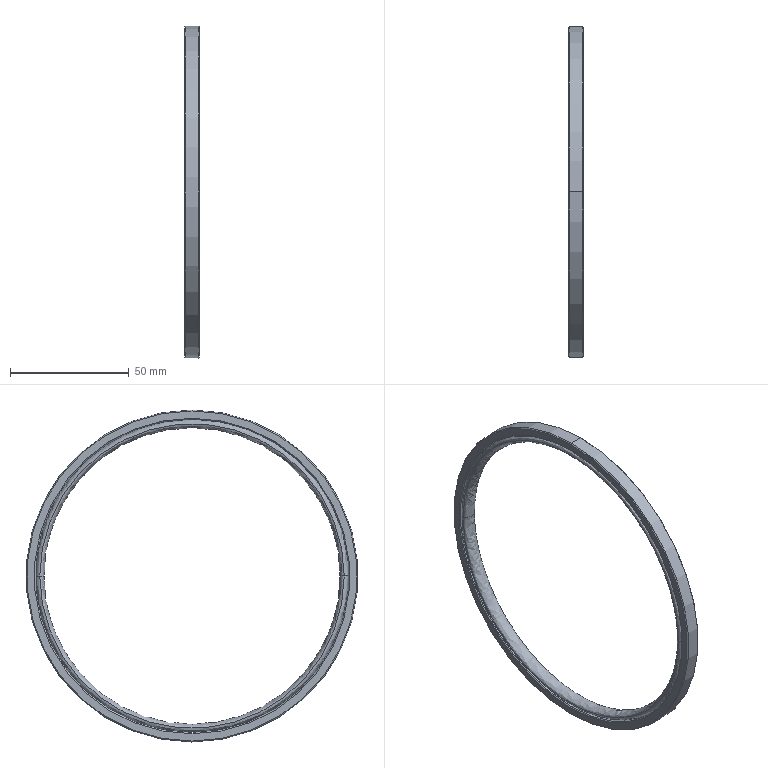Part | SolidWorks | features Revolution 3 | 2 solids | 18 faces | box 6.3 x 140 x 140 mm | volume 18044 mm3 | cone 8 | spline 4 | cylinder 4 | plane 2 | commonest cylinder face diameters 132.25 x2 140 x2
STEP:
#1=CARTESIAN_POINT('',(6.3,64.187,0.));
#2=VERTEX_POINT('',#1);
#3=CARTESIAN_POINT('',(6.3,-64.187,0.));
#4=VERTEX_POINT('',#3);
#5=CARTESIAN_POINT('',(6.3,0.,0.));
#6=DIRECTION('',(-1.,0.,0.));
#7=DIRECTION('',(0.,1.,0.));
#8=AXIS2_PLACEMENT_3D('',#5,#6,#7);
#9=CIRCLE('',#8,64.187);
#10=EDGE_CURVE('',#2,#4,#9,.T.);
#11=ORIENTED_EDGE('',*,*,#10,.T.);
#12=CARTESIAN_POINT('',(0.,-64.187,0.));
#13=VERTEX_POINT('',#12);
#14=CARTESIAN_POINT('',(6.3,-64.187,0.));
#15=CARTESIAN_POINT('',(6.3,-68.062,0.));
#16=CARTESIAN_POINT('',(0.,-68.062,0.));
#17=CARTESIAN_POINT('',(0.,-64.187,0.));
#18=(BOUNDED_CURVE()B_SPLINE_CURVE(3,(#14,#15,#16,#17),.UNSPECIFIED.,.F.,.T.)B_SPLINE_CURVE_WITH_KNOTS((4,4),(0.,3.142),.UNSPECIFIED.)CURVE()GEOMETRIC_REPRESENTATION_ITEM()RATIONAL_B_SPLINE_CURVE((1.,0.3333,0.3333,1.))REPRESENTATION_ITEM(''));
#19=EDGE_CURVE('',#4,#13,#18,.T.);
#20=ORIENTED_EDGE('',*,*,#19,.T.);
#21=CARTESIAN_POINT('',(0.,64.187,0.));
#22=VERTEX_POINT('',#21);
#23=CARTESIAN_POINT('',(0.,0.,0.));
#24=DIRECTION('',(-1.,0.,0.));
#25=DIRECTION('',(0.,1.,0.));
#26=AXIS2_PLACEMENT_3D('',#23,#24,#25);
#27=CIRCLE('',#26,64.187);
#28=EDGE_CURVE('',#22,#13,#27,.T.);
#29=ORIENTED_EDGE('',*,*,#28,.F.);
#30=CARTESIAN_POINT('',(6.3,64.187,0.));
#31=CARTESIAN_POINT('',(6.3,68.062,0.));
#32=CARTESIAN_POINT('',(0.,68.062,0.));
#33=CARTESIAN_POINT('',(0.,64.187,0.));
#34=(BOUNDED_CURVE()B_SPLINE_CURVE(3,(#30,#31,#32,#33),.UNSPECIFIED.,.F.,.F.)B_SPLINE_CURVE_WITH_KNOTS((4,4),(0.,3.142),.UNSPECIFIED.)CURVE()GEOMETRIC_REPRESENTATION_ITEM()RATIONAL_B_SPLINE_CURVE((1.,0.3333,0.3333,1.))REPRESENTATION_ITEM(''));
#35=EDGE_CURVE('',#2,#22,#34,.T.);
#36=ORIENTED_EDGE('',*,*,#35,.F.);
#37=EDGE_LOOP('',(#11,#20,#29,#36));
#38=FACE_OUTER_BOUND('',#37,.T.);
#39=CARTESIAN_POINT('',(6.3,64.187,0.));
#40=CARTESIAN_POINT('',(6.3,64.187,-128.375));
#41=CARTESIAN_POINT('',(6.3,-64.188,-128.375));
#42=CARTESIAN_POINT('',(6.3,-64.187,0.));
#43=CARTESIAN_POINT('',(6.3,68.062,0.));
#44=CARTESIAN_POINT('',(6.3,68.062,-136.125));
#45=CARTESIAN_POINT('',(6.3,-68.063,-136.125));
#46=CARTESIAN_POINT('',(6.3,-68.062,0.));
#47=CARTESIAN_POINT('',(0.,68.062,0.));
#48=CARTESIAN_POINT('',(0.,68.062,-136.125));
#49=CARTESIAN_POINT('',(0.,-68.063,-136.125));
#50=CARTESIAN_POINT('',(0.,-68.062,0.));
#51=CARTESIAN_POINT('',(0.,64.187,0.));
#52=CARTESIAN_POINT('',(0.,64.187,-128.375));
#53=CARTESIAN_POINT('',(0.,-64.188,-128.375));
#54=CARTESIAN_POINT('',(0.,-64.187,0.));
#55=(BOUNDED_SURFACE()B_SPLINE_SURFACE(3,3,((#39,#40,#41,#42),(#43,#44,#45,#46),(#47,#48,#49,#50),(#51,#52,#53,#54)),.UNSPECIFIED.,.F.,.F.,.F.)B_SPLINE_SURFACE_WITH_KNOTS((4,4),(4,4),(0.,1.),(0.,1.),.UNSPECIFIED.)GEOMETRIC_REPRESENTATION_ITEM()RATIONAL_B_SPLINE_SURFACE(((1.,0.3333,0.3333,1.),(0.3333,0.1111,0.1111,0.3333),(0.3333,0.1111,0.1111,0.3333),(1.,0.3333,0.3333,1.)))REPRESENTATION_ITEM('')SURFACE());
#56=ADVANCED_FACE('',(#38),#55,.F.);
#57=ORIENTED_EDGE('',*,*,#28,.T.);
#58=CARTESIAN_POINT('',(0.,-64.187,0.));
#59=CARTESIAN_POINT('',(0.,-60.312,0.));
#60=CARTESIAN_POINT('',(6.3,-60.312,0.));
#61=CARTESIAN_POINT('',(6.3,-64.187,0.));
#62=(BOUNDED_CURVE()B_SPLINE_CURVE(3,(#58,#59,#60,#61),.UNSPECIFIED.,.F.,.T.)B_SPLINE_CURVE_WITH_KNOTS((4,4),(3.142,6.283),.UNSPECIFIED.)CURVE()GEOMETRIC_REPRESENTATION_ITEM()RATIONAL_B_SPLINE_CURVE((1.,0.3333,0.3333,1.))REPRESENTATION_ITEM(''));
#63=EDGE_CURVE('',#13,#4,#62,.T.);
#64=ORIENTED_EDGE('',*,*,#63,.T.);
#65=ORIENTED_EDGE('',*,*,#10,.F.);
#66=CARTESIAN_POINT('',(0.,64.187,0.));
#67=CARTESIAN_POINT('',(0.,60.312,0.));
#68=CARTESIAN_POINT('',(6.3,60.312,0.));
#69=CARTESIAN_POINT('',(6.3,64.187,0.));
#70=(BOUNDED_CURVE()B_SPLINE_CURVE(3,(#66,#67,#68,#69),.UNSPECIFIED.,.F.,.T.)B_SPLINE_CURVE_WITH_KNOTS((4,4),(3.142,6.283),.UNSPECIFIED.)CURVE()GEOMETRIC_REPRESENTATION_ITEM()RATIONAL_B_SPLINE_CURVE((1.,0.3333,0.3333,1.))REPRESENTATION_ITEM(''));
#71=EDGE_CURVE('',#22,#2,#70,.T.);
#72=ORIENTED_EDGE('',*,*,#71,.F.);
#73=EDGE_LOOP('',(#57,#64,#65,#72));
#74=FACE_OUTER_BOUND('',#73,.T.);
#75=CARTESIAN_POINT('',(0.,64.187,0.));
#76=CARTESIAN_POINT('',(0.,64.187,-128.375));
#77=CARTESIAN_POINT('',(0.,-64.188,-128.375));
#78=CARTESIAN_POINT('',(0.,-64.187,0.));
#79=CARTESIAN_POINT('',(0.,60.312,0.));
#80=CARTESIAN_POINT('',(0.,60.312,-120.625));
#81=CARTESIAN_POINT('',(0.,-60.313,-120.625));
#82=CARTESIAN_POINT('',(0.,-60.312,0.));
#83=CARTESIAN_POINT('',(6.3,60.312,0.));
#84=CARTESIAN_POINT('',(6.3,60.312,-120.625));
#85=CARTESIAN_POINT('',(6.3,-60.313,-120.625));
#86=CARTESIAN_POINT('',(6.3,-60.312,0.));
#87=CARTESIAN_POINT('',(6.3,64.187,0.));
#88=CARTESIAN_POINT('',(6.3,64.187,-128.375));
#89=CARTESIAN_POINT('',(6.3,-64.188,-128.375));
#90=CARTESIAN_POINT('',(6.3,-64.187,0.));
#91=(BOUNDED_SURFACE()B_SPLINE_SURFACE(3,3,((#75,#76,#77,#78),(#79,#80,#81,#82),(#83,#84,#85,#86),(#87,#88,#89,#90)),.UNSPECIFIED.,.F.,.F.,.F.)B_SPLINE_SURFACE_WITH_KNOTS((4,4),(4,4),(0.,1.),(0.,1.),.UNSPECIFIED.)GEOMETRIC_REPRESENTATION_ITEM()RATIONAL_B_SPLINE_SURFACE(((1.,0.3333,0.3333,1.),(0.3333,0.1111,0.1111,0.3333),(0.3333,0.1111,0.1111,0.3333),(1.,0.3333,0.3333,1.)))REPRESENTATION_ITEM('')SURFACE());
#92=ADVANCED_FACE('',(#74),#91,.F.);
#93=ORIENTED_EDGE('',*,*,#63,.F.);
#94=CARTESIAN_POINT('',(0.,0.,0.));
#95=DIRECTION('',(-1.,0.,0.));
#96=DIRECTION('',(0.,1.,0.));
#97=AXIS2_PLACEMENT_3D('',#94,#95,#96);
#98=CIRCLE('',#97,64.187);
#99=EDGE_CURVE('',#13,#22,#98,.T.);
#100=ORIENTED_EDGE('',*,*,#99,.T.);
#101=ORIENTED_EDGE('',*,*,#71,.T.);
#102=CARTESIAN_POINT('',(6.3,0.,0.));
#103=DIRECTION('',(-1.,0.,0.));
#104=DIRECTION('',(0.,1.,0.));
#105=AXIS2_PLACEMENT_3D('',#102,#103,#104);
#106=CIRCLE('',#105,64.187);
#107=EDGE_CURVE('',#4,#2,#106,.T.);
#108=ORIENTED_EDGE('',*,*,#107,.F.);
#109=EDGE_LOOP('',(#93,#100,#101,#108));
#110=FACE_OUTER_BOUND('',#109,.T.);
#111=CARTESIAN_POINT('',(0.,-64.188,0.));
#112=CARTESIAN_POINT('',(0.,-64.187,128.375));
#113=CARTESIAN_POINT('',(0.,64.188,128.375));
#114=CARTESIAN_POINT('',(0.,64.188,0.));
#115=CARTESIAN_POINT('',(0.,-60.312,0.));
#116=CARTESIAN_POINT('',(0.,-60.312,120.625));
#117=CARTESIAN_POINT('',(0.,60.313,120.625));
#118=CARTESIAN_POINT('',(0.,60.312,0.));
#119=CARTESIAN_POINT('',(6.3,-60.312,0.));
#120=CARTESIAN_POINT('',(6.3,-60.312,120.625));
#121=CARTESIAN_POINT('',(6.3,60.313,120.625));
#122=CARTESIAN_POINT('',(6.3,60.312,0.));
#123=CARTESIAN_POINT('',(6.3,-64.187,0.));
#124=CARTESIAN_POINT('',(6.3,-64.187,128.375));
#125=CARTESIAN_POINT('',(6.3,64.188,128.375));
#126=CARTESIAN_POINT('',(6.3,64.187,0.));
#127=(BOUNDED_SURFACE()B_SPLINE_SURFACE(3,3,((#111,#112,#113,#114),(#115,#116,#117,#118),(#119,#120,#121,#122),(#123,#124,#125,#126)),.UNSPECIFIED.,.F.,.F.,.F.)B_SPLINE_SURFACE_WITH_KNOTS((4,4),(4,4),(0.,1.),(0.,1.),.UNSPECIFIED.)GEOMETRIC_REPRESENTATION_ITEM()RATIONAL_B_SPLINE_SURFACE(((1.,0.3333,0.3333,1.),(0.3333,0.1111,0.1111,0.3333),(0.3333,0.1111,0.1111,0.3333),(1.,0.3333,0.3333,1.)))REPRESENTATION_ITEM('')SURFACE());
#128=ADVANCED_FACE('',(#110),#127,.F.);
#129=ORIENTED_EDGE('',*,*,#19,.F.);
#130=ORIENTED_EDGE('',*,*,#107,.T.);
#131=ORIENTED_EDGE('',*,*,#35,.T.);
#132=ORIENTED_EDGE('',*,*,#99,.F.);
#133=EDGE_LOOP('',(#129,#130,#131,#132));
#134=FACE_OUTER_BOUND('',#133,.T.);
#135=CARTESIAN_POINT('',(6.3,-64.188,0.));
#136=CARTESIAN_POINT('',(6.3,-64.187,128.375));
#137=CARTESIAN_POINT('',(6.3,64.188,128.375));
#138=CARTESIAN_POINT('',(6.3,64.188,0.));
#139=CARTESIAN_POINT('',(6.3,-68.062,0.));
#140=CARTESIAN_POINT('',(6.3,-68.062,136.125));
#141=CARTESIAN_POINT('',(6.3,68.063,136.125));
#142=CARTESIAN_POINT('',(6.3,68.062,0.));
#143=CARTESIAN_POINT('',(0.,-68.062,0.));
#144=CARTESIAN_POINT('',(0.,-68.062,136.125));
#145=CARTESIAN_POINT('',(0.,68.063,136.125));
#146=CARTESIAN_POINT('',(0.,68.062,0.));
#147=CARTESIAN_POINT('',(0.,-64.188,0.));
#148=CARTESIAN_POINT('',(0.,-64.187,128.375));
#149=CARTESIAN_POINT('',(0.,64.188,128.375));
#150=CARTESIAN_POINT('',(0.,64.188,0.));
#151=(BOUNDED_SURFACE()B_SPLINE_SURFACE(3,3,((#135,#136,#137,#138),(#139,#140,#141,#142),(#143,#144,#145,#146),(#147,#148,#149,#150)),.UNSPECIFIED.,.F.,.F.,.F.)B_SPLINE_SURFACE_WITH_KNOTS((4,4),(4,4),(0.,1.),(0.,1.),.UNSPECIFIED.)GEOMETRIC_REPRESENTATION_ITEM()RATIONAL_B_SPLINE_SURFACE(((1.,0.3333,0.3333,1.),(0.3333,0.1111,0.1111,0.3333),(0.3333,0.1111,0.1111,0.3333),(1.,0.3333,0.3333,1.)))REPRESENTATION_ITEM('')SURFACE());
#152=ADVANCED_FACE('',(#134),#151,.F.);
#153=CLOSED_SHELL('',(#56,#92,#128,#152));
#154=MANIFOLD_SOLID_BREP('',#153);
#155=CARTESIAN_POINT('',(0.3875,0.,-66.125));
#156=VERTEX_POINT('',#155);
#157=CARTESIAN_POINT('',(0.3875,0.,66.125));
#158=VERTEX_POINT('',#157);
#159=CARTESIAN_POINT('',(0.3875,0.,0.));
#160=DIRECTION('',(-1.,0.,0.));
#161=DIRECTION('',(0.,0.,1.));
#162=AXIS2_PLACEMENT_3D('',#159,#160,#161);
#163=CIRCLE('',#162,66.125);
#164=EDGE_CURVE('',#156,#158,#163,.T.);
#165=ORIENTED_EDGE('',*,*,#164,.F.);
#166=CARTESIAN_POINT('',(0.,0.,-66.512));
#167=VERTEX_POINT('',#166);
#168=CARTESIAN_POINT('',(0.,0.,-66.513));
#169=DIRECTION('',(-0.7071,0.,-0.7071));
#170=VECTOR('',#169,1000.);
#171=LINE('',#168,#170);
#172=EDGE_CURVE('',#156,#167,#171,.T.);
#173=ORIENTED_EDGE('',*,*,#172,.T.);
#174=CARTESIAN_POINT('',(0.,0.,66.513));
#175=VERTEX_POINT('',#174);
#176=CARTESIAN_POINT('',(0.,0.,0.));
#177=DIRECTION('',(-1.,0.,0.));
#178=DIRECTION('',(0.,0.,1.));
#179=AXIS2_PLACEMENT_3D('',#176,#177,#178);
#180=CIRCLE('',#179,66.513);
#181=EDGE_CURVE('',#167,#175,#180,.T.);
#182=ORIENTED_EDGE('',*,*,#181,.T.);
#183=CARTESIAN_POINT('',(0.,0.,66.513));
#184=DIRECTION('',(-0.7071,0.,0.7071));
#185=VECTOR('',#184,1000.);
#186=LINE('',#183,#185);
#187=EDGE_CURVE('',#158,#175,#186,.T.);
#188=ORIENTED_EDGE('',*,*,#187,.F.);
#189=EDGE_LOOP('',(#165,#173,#182,#188));
#190=FACE_OUTER_BOUND('',#189,.T.);
#191=CARTESIAN_POINT('',(0.,0.,0.));
#192=DIRECTION('',(-1.,0.,0.));
#193=DIRECTION('',(0.,0.,1.));
#194=AXIS2_PLACEMENT_3D('',#191,#192,#193);
#195=CONICAL_SURFACE('',#194,66.513,0.7854);
#196=ADVANCED_FACE('',(#190),#195,.F.);
#197=CARTESIAN_POINT('',(0.,0.,69.612));
#198=VERTEX_POINT('',#197);
#199=CARTESIAN_POINT('',(0.,0.,-69.612));
#200=VERTEX_POINT('',#199);
#201=CARTESIAN_POINT('',(0.,0.,0.));
#202=DIRECTION('',(-1.,0.,0.));
#203=DIRECTION('',(0.,0.,1.));
#204=AXIS2_PLACEMENT_3D('',#201,#202,#203);
#205=CIRCLE('',#204,69.613);
#206=EDGE_CURVE('',#198,#200,#205,.T.);
#207=ORIENTED_EDGE('',*,*,#206,.F.);
#208=CARTESIAN_POINT('',(0.3875,0.,70.));
#209=VERTEX_POINT('',#208);
#210=CARTESIAN_POINT('',(0.3875,0.,70.));
#211=DIRECTION('',(0.7071,0.,0.7071));
#212=VECTOR('',#211,1000.);
#213=LINE('',#210,#212);
#214=EDGE_CURVE('',#198,#209,#213,.T.);
#215=ORIENTED_EDGE('',*,*,#214,.T.);
#216=CARTESIAN_POINT('',(0.3875,0.,-70.));
#217=VERTEX_POINT('',#216);
#218=CARTESIAN_POINT('',(0.3875,0.,0.));
#219=DIRECTION('',(-1.,0.,0.));
#220=DIRECTION('',(0.,0.,1.));
#221=AXIS2_PLACEMENT_3D('',#218,#219,#220);
#222=CIRCLE('',#221,70.);
#223=EDGE_CURVE('',#209,#217,#222,.T.);
#224=ORIENTED_EDGE('',*,*,#223,.T.);
#225=CARTESIAN_POINT('',(0.3875,0.,-70.));
#226=DIRECTION('',(0.7071,0.,-0.7071));
#227=VECTOR('',#226,1000.);
#228=LINE('',#225,#227);
#229=EDGE_CURVE('',#200,#217,#228,.T.);
#230=ORIENTED_EDGE('',*,*,#229,.F.);
#231=EDGE_LOOP('',(#207,#215,#224,#230));
#232=FACE_OUTER_BOUND('',#231,.T.);
#233=CARTESIAN_POINT('',(0.3875,0.,0.));
#234=DIRECTION('',(1.,0.,0.));
#235=DIRECTION('',(0.,0.,-1.));
#236=AXIS2_PLACEMENT_3D('',#233,#234,#235);
#237=CONICAL_SURFACE('',#236,70.,0.7854);
#238=ADVANCED_FACE('',(#232),#237,.T.);
#239=CARTESIAN_POINT('',(5.912,0.,70.));
#240=VERTEX_POINT('',#239);
#241=CARTESIAN_POINT('',(5.912,0.,-70.));
#242=VERTEX_POINT('',#241);
#243=CARTESIAN_POINT('',(5.912,0.,0.));
#244=DIRECTION('',(-1.,0.,0.));
#245=DIRECTION('',(0.,0.,1.));
#246=AXIS2_PLACEMENT_3D('',#243,#244,#245);
#247=CIRCLE('',#246,70.);
#248=EDGE_CURVE('',#240,#242,#247,.T.);
#249=ORIENTED_EDGE('',*,*,#248,.T.);
#250=CARTESIAN_POINT('',(0.,0.,-70.));
#251=DIRECTION('',(-1.,0.,0.));
#252=VECTOR('',#251,1000.);
#253=LINE('',#250,#252);
#254=EDGE_CURVE('',#242,#217,#253,.T.);
#255=ORIENTED_EDGE('',*,*,#254,.T.);
#256=ORIENTED_EDGE('',*,*,#223,.F.);
#257=CARTESIAN_POINT('',(0.,0.,70.));
#258=DIRECTION('',(-1.,0.,0.));
#259=VECTOR('',#258,1000.);
#260=LINE('',#257,#259);
#261=EDGE_CURVE('',#240,#209,#260,.T.);
#262=ORIENTED_EDGE('',*,*,#261,.F.);
#263=EDGE_LOOP('',(#249,#255,#256,#262));
#264=FACE_OUTER_BOUND('',#263,.T.);
#265=CARTESIAN_POINT('',(0.,0.,0.));
#266=DIRECTION('',(-1.,0.,0.));
#267=DIRECTION('',(0.,0.,1.));
#268=AXIS2_PLACEMENT_3D('',#265,#266,#267);
#269=CYLINDRICAL_SURFACE('',#268,70.);
#270=ADVANCED_FACE('',(#264),#269,.T.);
#271=CARTESIAN_POINT('',(6.3,0.,69.612));
#272=VERTEX_POINT('',#271);
#273=CARTESIAN_POINT('',(6.3,0.,-69.613));
#274=VERTEX_POINT('',#273);
#275=CARTESIAN_POINT('',(6.3,0.,0.));
#276=DIRECTION('',(-1.,0.,0.));
#277=DIRECTION('',(0.,0.,1.));
#278=AXIS2_PLACEMENT_3D('',#275,#276,#277);
#279=CIRCLE('',#278,69.613);
#280=EDGE_CURVE('',#272,#274,#279,.T.);
#281=ORIENTED_EDGE('',*,*,#280,.T.);
#282=CARTESIAN_POINT('',(5.912,0.,-70.));
#283=DIRECTION('',(-0.7071,0.,-0.7071));
#284=VECTOR('',#283,1000.);
#285=LINE('',#282,#284);
#286=EDGE_CURVE('',#274,#242,#285,.T.);
#287=ORIENTED_EDGE('',*,*,#286,.T.);
#288=ORIENTED_EDGE('',*,*,#248,.F.);
#289=CARTESIAN_POINT('',(5.912,0.,70.));
#290=DIRECTION('',(-0.7071,0.,0.7071));
#291=VECTOR('',#290,1000.);
#292=LINE('',#289,#291);
#293=EDGE_CURVE('',#272,#240,#292,.T.);
#294=ORIENTED_EDGE('',*,*,#293,.F.);
#295=EDGE_LOOP('',(#281,#287,#288,#294));
#296=FACE_OUTER_BOUND('',#295,.T.);
#297=CARTESIAN_POINT('',(5.912,0.,0.));
#298=DIRECTION('',(-1.,0.,0.));
#299=DIRECTION('',(0.,0.,1.));
#300=AXIS2_PLACEMENT_3D('',#297,#298,#299);
#301=CONICAL_SURFACE('',#300,70.,0.7854);
#302=ADVANCED_FACE('',(#296),#301,.T.);
#303=CARTESIAN_POINT('',(5.912,0.,-66.125));
#304=VERTEX_POINT('',#303);
#305=CARTESIAN_POINT('',(5.912,0.,66.125));
#306=VERTEX_POINT('',#305);
#307=CARTESIAN_POINT('',(5.912,0.,0.));
#308=DIRECTION('',(-1.,0.,0.));
#309=DIRECTION('',(0.,0.,1.));
#310=AXIS2_PLACEMENT_3D('',#307,#308,#309);
#311=CIRCLE('',#310,66.125);
#312=EDGE_CURVE('',#304,#306,#311,.T.);
#313=ORIENTED_EDGE('',*,*,#312,.T.);
#314=CARTESIAN_POINT('',(6.3,0.,66.512));
#315=VERTEX_POINT('',#314);
#316=CARTESIAN_POINT('',(5.912,0.,66.125));
#317=DIRECTION('',(0.7071,0.,0.7071));
#318=VECTOR('',#317,1000.);
#319=LINE('',#316,#318);
#320=EDGE_CURVE('',#306,#315,#319,.T.);
#321=ORIENTED_EDGE('',*,*,#320,.T.);
#322=CARTESIAN_POINT('',(6.3,0.,-66.513));
#323=VERTEX_POINT('',#322);
#324=CARTESIAN_POINT('',(6.3,0.,0.));
#325=DIRECTION('',(-1.,0.,0.));
#326=DIRECTION('',(0.,0.,1.));
#327=AXIS2_PLACEMENT_3D('',#324,#325,#326);
#328=CIRCLE('',#327,66.513);
#329=EDGE_CURVE('',#323,#315,#328,.T.);
#330=ORIENTED_EDGE('',*,*,#329,.F.);
#331=CARTESIAN_POINT('',(5.912,0.,-66.125));
#332=DIRECTION('',(0.7071,0.,-0.7071));
#333=VECTOR('',#332,1000.);
#334=LINE('',#331,#333);
#335=EDGE_CURVE('',#304,#323,#334,.T.);
#336=ORIENTED_EDGE('',*,*,#335,.F.);
#337=EDGE_LOOP('',(#313,#321,#330,#336));
#338=FACE_OUTER_BOUND('',#337,.T.);
#339=CARTESIAN_POINT('',(5.912,0.,0.));
#340=DIRECTION('',(1.,0.,0.));
#341=DIRECTION('',(0.,0.,-1.));
#342=AXIS2_PLACEMENT_3D('',#339,#340,#341);
#343=CONICAL_SURFACE('',#342,66.125,0.7854);
#344=ADVANCED_FACE('',(#338),#343,.F.);
#345=ORIENTED_EDGE('',*,*,#312,.F.);
#346=CARTESIAN_POINT('',(0.,0.,-66.125));
#347=DIRECTION('',(-1.,0.,0.));
#348=VECTOR('',#347,1000.);
#349=LINE('',#346,#348);
#350=EDGE_CURVE('',#304,#156,#349,.T.);
#351=ORIENTED_EDGE('',*,*,#350,.T.);
#352=ORIENTED_EDGE('',*,*,#164,.T.);
#353=CARTESIAN_POINT('',(0.,0.,66.125));
#354=DIRECTION('',(-1.,0.,0.));
#355=VECTOR('',#354,1000.);
#356=LINE('',#353,#355);
#357=EDGE_CURVE('',#306,#158,#356,.T.);
#358=ORIENTED_EDGE('',*,*,#357,.F.);
#359=EDGE_LOOP('',(#345,#351,#352,#358));
#360=FACE_OUTER_BOUND('',#359,.T.);
#361=CARTESIAN_POINT('',(0.,0.,0.));
#362=DIRECTION('',(-1.,0.,0.));
#363=DIRECTION('',(0.,0.,1.));
#364=AXIS2_PLACEMENT_3D('',#361,#362,#363);
#365=CYLINDRICAL_SURFACE('',#364,66.125);
#366=ADVANCED_FACE('',(#360),#365,.F.);
#367=ORIENTED_EDGE('',*,*,#350,.F.);
#368=CARTESIAN_POINT('',(5.912,0.,0.));
#369=DIRECTION('',(-1.,0.,0.));
#370=DIRECTION('',(0.,0.,1.));
#371=AXIS2_PLACEMENT_3D('',#368,#369,#370);
#372=CIRCLE('',#371,66.125);
#373=EDGE_CURVE('',#306,#304,#372,.T.);
#374=ORIENTED_EDGE('',*,*,#373,.F.);
#375=ORIENTED_EDGE('',*,*,#357,.T.);
#376=CARTESIAN_POINT('',(0.3875,0.,0.));
#377=DIRECTION('',(-1.,0.,0.));
#378=DIRECTION('',(0.,0.,1.));
#379=AXIS2_PLACEMENT_3D('',#376,#377,#378);
#380=CIRCLE('',#379,66.125);
#381=EDGE_CURVE('',#158,#156,#380,.T.);
#382=ORIENTED_EDGE('',*,*,#381,.T.);
#383=EDGE_LOOP('',(#367,#374,#375,#382));
#384=FACE_OUTER_BOUND('',#383,.T.);
#385=CARTESIAN_POINT('',(0.,0.,0.));
#386=DIRECTION('',(-1.,0.,0.));
#387=DIRECTION('',(0.,0.,1.));
#388=AXIS2_PLACEMENT_3D('',#385,#386,#387);
#389=CYLINDRICAL_SURFACE('',#388,66.125);
#390=ADVANCED_FACE('',(#384),#389,.F.);
#391=ORIENTED_EDGE('',*,*,#320,.F.);
#392=ORIENTED_EDGE('',*,*,#373,.T.);
#393=ORIENTED_EDGE('',*,*,#335,.T.);
#394=CARTESIAN_POINT('',(6.3,0.,0.));
#395=DIRECTION('',(-1.,0.,0.));
#396=DIRECTION('',(0.,0.,1.));
#397=AXIS2_PLACEMENT_3D('',#394,#395,#396);
#398=CIRCLE('',#397,66.513);
#399=EDGE_CURVE('',#315,#323,#398,.T.);
#400=ORIENTED_EDGE('',*,*,#399,.F.);
#401=EDGE_LOOP('',(#391,#392,#393,#400));
#402=FACE_OUTER_BOUND('',#401,.T.);
#403=CARTESIAN_POINT('',(5.912,0.,0.));
#404=DIRECTION('',(1.,0.,0.));
#405=DIRECTION('',(0.,0.,-1.));
#406=AXIS2_PLACEMENT_3D('',#403,#404,#405);
#407=CONICAL_SURFACE('',#406,66.125,0.7854);
#408=ADVANCED_FACE('',(#402),#407,.F.);
#409=ORIENTED_EDGE('',*,*,#329,.T.);
#410=ORIENTED_EDGE('',*,*,#399,.T.);
#411=EDGE_LOOP('',(#409,#410));
#412=FACE_BOUND('',#411,.T.);
#413=ORIENTED_EDGE('',*,*,#280,.F.);
#414=CARTESIAN_POINT('',(6.3,0.,0.));
#415=DIRECTION('',(-1.,0.,0.));
#416=DIRECTION('',(0.,0.,1.));
#417=AXIS2_PLACEMENT_3D('',#414,#415,#416);
#418=CIRCLE('',#417,69.613);
#419=EDGE_CURVE('',#274,#272,#418,.T.);
#420=ORIENTED_EDGE('',*,*,#419,.F.);
#421=EDGE_LOOP('',(#413,#420));
#422=FACE_OUTER_BOUND('',#421,.T.);
#423=CARTESIAN_POINT('',(6.3,0.,0.));
#424=DIRECTION('',(1.,0.,0.));
#425=DIRECTION('',(0.,0.,-1.));
#426=AXIS2_PLACEMENT_3D('',#423,#424,#425);
#427=PLANE('',#426);
#428=ADVANCED_FACE('',(#412,#422),#427,.T.);
#429=ORIENTED_EDGE('',*,*,#286,.F.);
#430=ORIENTED_EDGE('',*,*,#419,.T.);
#431=ORIENTED_EDGE('',*,*,#293,.T.);
#432=CARTESIAN_POINT('',(5.912,0.,0.));
#433=DIRECTION('',(-1.,0.,0.));
#434=DIRECTION('',(0.,0.,1.));
#435=AXIS2_PLACEMENT_3D('',#432,#433,#434);
#436=CIRCLE('',#435,70.);
#437=EDGE_CURVE('',#242,#240,#436,.T.);
#438=ORIENTED_EDGE('',*,*,#437,.F.);
#439=EDGE_LOOP('',(#429,#430,#431,#438));
#440=FACE_OUTER_BOUND('',#439,.T.);
#441=CARTESIAN_POINT('',(5.912,0.,0.));
#442=DIRECTION('',(-1.,0.,0.));
#443=DIRECTION('',(0.,0.,1.));
#444=AXIS2_PLACEMENT_3D('',#441,#442,#443);
#445=CONICAL_SURFACE('',#444,70.,0.7854);
#446=ADVANCED_FACE('',(#440),#445,.T.);
#447=ORIENTED_EDGE('',*,*,#254,.F.);
#448=ORIENTED_EDGE('',*,*,#437,.T.);
#449=ORIENTED_EDGE('',*,*,#261,.T.);
#450=CARTESIAN_POINT('',(0.3875,0.,0.));
#451=DIRECTION('',(-1.,0.,0.));
#452=DIRECTION('',(0.,0.,1.));
#453=AXIS2_PLACEMENT_3D('',#450,#451,#452);
#454=CIRCLE('',#453,70.);
#455=EDGE_CURVE('',#217,#209,#454,.T.);
#456=ORIENTED_EDGE('',*,*,#455,.F.);
#457=EDGE_LOOP('',(#447,#448,#449,#456));
#458=FACE_OUTER_BOUND('',#457,.T.);
#459=CARTESIAN_POINT('',(0.,0.,0.));
#460=DIRECTION('',(-1.,0.,0.));
#461=DIRECTION('',(0.,0.,1.));
#462=AXIS2_PLACEMENT_3D('',#459,#460,#461);
#463=CYLINDRICAL_SURFACE('',#462,70.);
#464=ADVANCED_FACE('',(#458),#463,.T.);
#465=ORIENTED_EDGE('',*,*,#214,.F.);
#466=CARTESIAN_POINT('',(0.,0.,0.));
#467=DIRECTION('',(-1.,0.,0.));
#468=DIRECTION('',(0.,0.,1.));
#469=AXIS2_PLACEMENT_3D('',#466,#467,#468);
#470=CIRCLE('',#469,69.613);
#471=EDGE_CURVE('',#200,#198,#470,.T.);
#472=ORIENTED_EDGE('',*,*,#471,.F.);
#473=ORIENTED_EDGE('',*,*,#229,.T.);
#474=ORIENTED_EDGE('',*,*,#455,.T.);
#475=EDGE_LOOP('',(#465,#472,#473,#474));
#476=FACE_OUTER_BOUND('',#475,.T.);
#477=CARTESIAN_POINT('',(0.3875,0.,0.));
#478=DIRECTION('',(1.,0.,0.));
#479=DIRECTION('',(0.,0.,-1.));
#480=AXIS2_PLACEMENT_3D('',#477,#478,#479);
#481=CONICAL_SURFACE('',#480,70.,0.7854);
#482=ADVANCED_FACE('',(#476),#481,.T.);
#483=ORIENTED_EDGE('',*,*,#471,.T.);
#484=ORIENTED_EDGE('',*,*,#206,.T.);
#485=EDGE_LOOP('',(#483,#484));
#486=FACE_OUTER_BOUND('',#485,.T.);
#487=CARTESIAN_POINT('',(0.,0.,0.));
#488=DIRECTION('',(-1.,0.,0.));
#489=DIRECTION('',(0.,0.,1.));
#490=AXIS2_PLACEMENT_3D('',#487,#488,#489);
#491=CIRCLE('',#490,66.513);
#492=EDGE_CURVE('',#175,#167,#491,.T.);
#493=ORIENTED_EDGE('',*,*,#492,.F.);
#494=ORIENTED_EDGE('',*,*,#181,.F.);
#495=EDGE_LOOP('',(#493,#494));
#496=FACE_BOUND('',#495,.T.);
#497=CARTESIAN_POINT('',(0.,0.,0.));
#498=DIRECTION('',(-1.,0.,0.));
#499=DIRECTION('',(0.,0.,1.));
#500=AXIS2_PLACEMENT_3D('',#497,#498,#499);
#501=PLANE('',#500);
#502=ADVANCED_FACE('',(#486,#496),#501,.T.);
#503=ORIENTED_EDGE('',*,*,#172,.F.);
#504=ORIENTED_EDGE('',*,*,#381,.F.);
#505=ORIENTED_EDGE('',*,*,#187,.T.);
#506=ORIENTED_EDGE('',*,*,#492,.T.);
#507=EDGE_LOOP('',(#503,#504,#505,#506));
#508=FACE_OUTER_BOUND('',#507,.T.);
#509=CARTESIAN_POINT('',(0.,0.,0.));
#510=DIRECTION('',(-1.,0.,0.));
#511=DIRECTION('',(0.,0.,1.));
#512=AXIS2_PLACEMENT_3D('',#509,#510,#511);
#513=CONICAL_SURFACE('',#512,66.513,0.7854);
#514=ADVANCED_FACE('',(#508),#513,.F.);
#515=CLOSED_SHELL('',(#196,#238,#270,#302,#344,#366,#390,#408,#428,#446,#464,#482,#502,#514));
#516=MANIFOLD_SOLID_BREP('',#515);
#517=CARTESIAN_POINT('',(0.,0.,0.));
#518=DIRECTION('',(0.,0.,1.));
#519=DIRECTION('',(1.,0.,0.));
#520=AXIS2_PLACEMENT_3D('',#517,#518,#519);
#521=(LENGTH_UNIT()NAMED_UNIT(*)SI_UNIT(.MILLI.,.METRE.));
#522=UNCERTAINTY_MEASURE_WITH_UNIT(LENGTH_MEASURE(0.00001),#521,'','');
#523=(NAMED_UNIT(*)PLANE_ANGLE_UNIT()SI_UNIT($,.RADIAN.));
#524=(NAMED_UNIT(*)SI_UNIT($,.STERADIAN.)SOLID_ANGLE_UNIT());
#525=(GEOMETRIC_REPRESENTATION_CONTEXT(3)GLOBAL_UNCERTAINTY_ASSIGNED_CONTEXT((#522))GLOBAL_UNIT_ASSIGNED_CONTEXT((#521,#523,#524))REPRESENTATION_CONTEXT('',''));
#526=ADVANCED_BREP_SHAPE_REPRESENTATION('',(#154,#516,#520),#525);